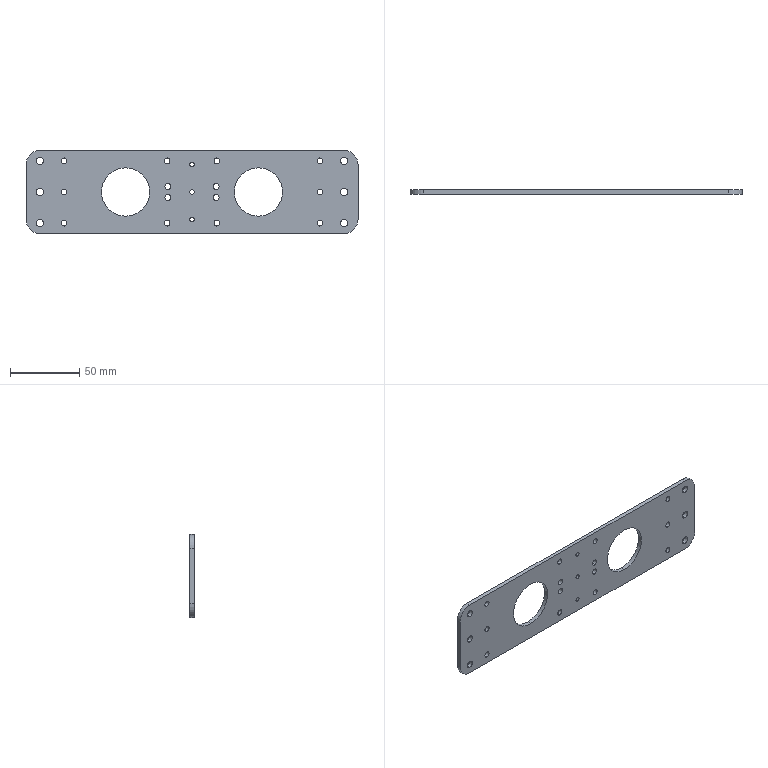Part | SolidWorks | features BaseBody 1 | 1 solid | 60 faces | box 240 x 3 x 60 mm | volume 36133 mm3 | cylinder 54 | plane 6 | commonest cylinder face diameters 4.2 x28 5.2 x12 3.2 x6 20 x4 35 x4